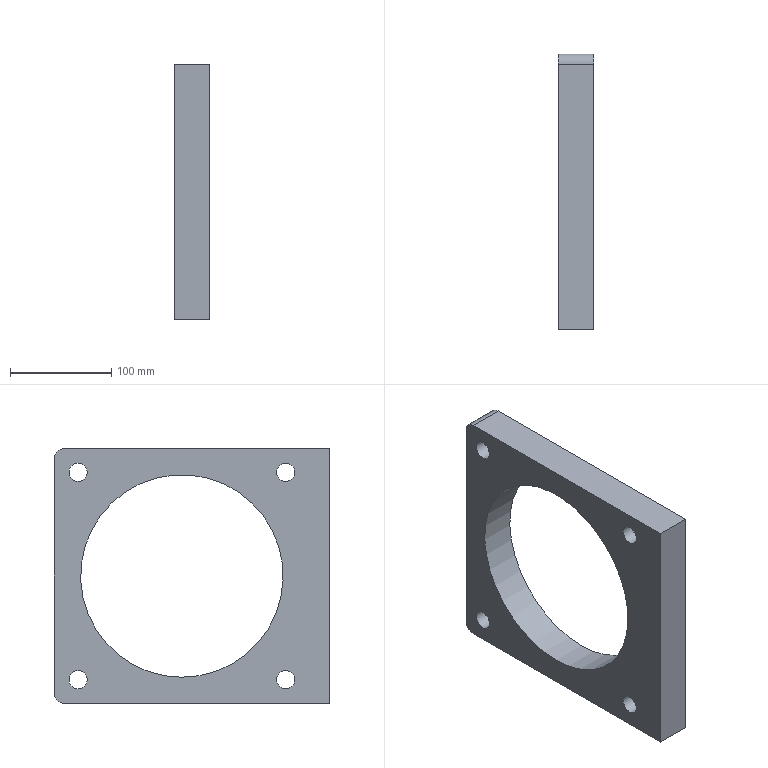Part | NX | features BREP 1, DATUM_CSYS 1 | 1 solid | 13 faces | box 35 x 272 x 252 mm | volume 1262355 mm3 | cylinder 7 | plane 6 | commonest cylinder face diameters 18 x4 20 x2 200 x1
STEP:
#1=CARTESIAN_POINT('',(-284.,116.,126.));
#2=VERTEX_POINT('',#1);
#3=CARTESIAN_POINT('',(-284.,-146.,126.));
#4=VERTEX_POINT('',#3);
#5=CARTESIAN_POINT('',(-284.,126.,126.));
#6=DIRECTION('',(0.,-1.,0.));
#7=VECTOR('',#6,1000.);
#8=LINE('',#5,#7);
#9=EDGE_CURVE('',#2,#4,#8,.T.);
#10=ORIENTED_EDGE('',*,*,#9,.F.);
#11=CARTESIAN_POINT('',(-319.,116.,126.));
#12=VERTEX_POINT('',#11);
#13=CARTESIAN_POINT('',(-284.,116.,126.));
#14=DIRECTION('',(-1.,0.,0.));
#15=VECTOR('',#14,1000.);
#16=LINE('',#13,#15);
#17=EDGE_CURVE('',#2,#12,#16,.T.);
#18=ORIENTED_EDGE('',*,*,#17,.T.);
#19=CARTESIAN_POINT('',(-319.,-146.,126.));
#20=VERTEX_POINT('',#19);
#21=CARTESIAN_POINT('',(-319.,126.,126.));
#22=DIRECTION('',(0.,-1.,0.));
#23=VECTOR('',#22,1000.);
#24=LINE('',#21,#23);
#25=EDGE_CURVE('',#12,#20,#24,.T.);
#26=ORIENTED_EDGE('',*,*,#25,.T.);
#27=CARTESIAN_POINT('',(-284.,-146.,126.));
#28=DIRECTION('',(-1.,0.,0.));
#29=VECTOR('',#28,1000.);
#30=LINE('',#27,#29);
#31=EDGE_CURVE('',#4,#20,#30,.T.);
#32=ORIENTED_EDGE('',*,*,#31,.F.);
#33=EDGE_LOOP('',(#10,#18,#26,#32));
#34=FACE_BOUND('',#33,.T.);
#35=CARTESIAN_POINT('',(-284.,126.,126.));
#36=DIRECTION('',(0.,0.,-1.));
#37=DIRECTION('',(0.,1.,0.));
#38=AXIS2_PLACEMENT_3D('',#35,#36,#37);
#39=PLANE('',#38);
#40=ADVANCED_FACE('',(#34),#39,.F.);
#41=CARTESIAN_POINT('',(-319.,-146.,-126.));
#42=VERTEX_POINT('',#41);
#43=CARTESIAN_POINT('',(-319.,-146.,126.));
#44=DIRECTION('',(0.,0.,-1.));
#45=VECTOR('',#44,1000.);
#46=LINE('',#43,#45);
#47=EDGE_CURVE('',#20,#42,#46,.T.);
#48=ORIENTED_EDGE('',*,*,#47,.T.);
#49=CARTESIAN_POINT('',(-284.,-146.,-126.));
#50=VERTEX_POINT('',#49);
#51=CARTESIAN_POINT('',(-284.,-146.,-126.));
#52=DIRECTION('',(-1.,0.,0.));
#53=VECTOR('',#52,1000.);
#54=LINE('',#51,#53);
#55=EDGE_CURVE('',#50,#42,#54,.T.);
#56=ORIENTED_EDGE('',*,*,#55,.F.);
#57=CARTESIAN_POINT('',(-284.,-146.,126.));
#58=DIRECTION('',(0.,0.,-1.));
#59=VECTOR('',#58,1000.);
#60=LINE('',#57,#59);
#61=EDGE_CURVE('',#4,#50,#60,.T.);
#62=ORIENTED_EDGE('',*,*,#61,.F.);
#63=ORIENTED_EDGE('',*,*,#31,.T.);
#64=EDGE_LOOP('',(#48,#56,#62,#63));
#65=FACE_BOUND('',#64,.T.);
#66=CARTESIAN_POINT('',(-284.,-146.,126.));
#67=DIRECTION('',(0.,1.,0.));
#68=DIRECTION('',(0.,0.,1.));
#69=AXIS2_PLACEMENT_3D('',#66,#67,#68);
#70=PLANE('',#69);
#71=ADVANCED_FACE('',(#65),#70,.F.);
#72=CARTESIAN_POINT('',(-319.,116.,-126.));
#73=VERTEX_POINT('',#72);
#74=CARTESIAN_POINT('',(-319.,-146.,-126.));
#75=DIRECTION('',(0.,1.,0.));
#76=VECTOR('',#75,1000.);
#77=LINE('',#74,#76);
#78=EDGE_CURVE('',#42,#73,#77,.T.);
#79=ORIENTED_EDGE('',*,*,#78,.T.);
#80=CARTESIAN_POINT('',(-284.,116.,-126.));
#81=VERTEX_POINT('',#80);
#82=CARTESIAN_POINT('',(-284.,116.,-126.));
#83=DIRECTION('',(-1.,0.,0.));
#84=VECTOR('',#83,1000.);
#85=LINE('',#82,#84);
#86=EDGE_CURVE('',#73,#81,#85,.F.);
#87=ORIENTED_EDGE('',*,*,#86,.T.);
#88=CARTESIAN_POINT('',(-284.,-146.,-126.));
#89=DIRECTION('',(0.,1.,0.));
#90=VECTOR('',#89,1000.);
#91=LINE('',#88,#90);
#92=EDGE_CURVE('',#50,#81,#91,.T.);
#93=ORIENTED_EDGE('',*,*,#92,.F.);
#94=ORIENTED_EDGE('',*,*,#55,.T.);
#95=EDGE_LOOP('',(#79,#87,#93,#94));
#96=FACE_BOUND('',#95,.T.);
#97=CARTESIAN_POINT('',(-284.,-146.,-126.));
#98=DIRECTION('',(0.,0.,1.));
#99=DIRECTION('',(1.,0.,0.));
#100=AXIS2_PLACEMENT_3D('',#97,#98,#99);
#101=PLANE('',#100);
#102=ADVANCED_FACE('',(#96),#101,.F.);
#103=CARTESIAN_POINT('',(-284.,126.,-116.));
#104=VERTEX_POINT('',#103);
#105=CARTESIAN_POINT('',(-284.,126.,116.));
#106=VERTEX_POINT('',#105);
#107=CARTESIAN_POINT('',(-284.,126.,-126.));
#108=DIRECTION('',(0.,0.,1.));
#109=VECTOR('',#108,1000.);
#110=LINE('',#107,#109);
#111=EDGE_CURVE('',#104,#106,#110,.T.);
#112=ORIENTED_EDGE('',*,*,#111,.F.);
#113=CARTESIAN_POINT('',(-319.,126.,-116.));
#114=VERTEX_POINT('',#113);
#115=CARTESIAN_POINT('',(-284.,126.,-116.));
#116=DIRECTION('',(-1.,0.,0.));
#117=VECTOR('',#116,1000.);
#118=LINE('',#115,#117);
#119=EDGE_CURVE('',#104,#114,#118,.T.);
#120=ORIENTED_EDGE('',*,*,#119,.T.);
#121=CARTESIAN_POINT('',(-319.,126.,116.));
#122=VERTEX_POINT('',#121);
#123=CARTESIAN_POINT('',(-319.,126.,-126.));
#124=DIRECTION('',(0.,0.,1.));
#125=VECTOR('',#124,1000.);
#126=LINE('',#123,#125);
#127=EDGE_CURVE('',#114,#122,#126,.T.);
#128=ORIENTED_EDGE('',*,*,#127,.T.);
#129=CARTESIAN_POINT('',(-284.,126.,116.));
#130=DIRECTION('',(-1.,0.,0.));
#131=VECTOR('',#130,1000.);
#132=LINE('',#129,#131);
#133=EDGE_CURVE('',#122,#106,#132,.F.);
#134=ORIENTED_EDGE('',*,*,#133,.T.);
#135=EDGE_LOOP('',(#112,#120,#128,#134));
#136=FACE_BOUND('',#135,.T.);
#137=CARTESIAN_POINT('',(-284.,126.,-126.));
#138=DIRECTION('',(0.,-1.,0.));
#139=DIRECTION('',(0.,0.,-1.));
#140=AXIS2_PLACEMENT_3D('',#137,#138,#139);
#141=PLANE('',#140);
#142=ADVANCED_FACE('',(#136),#141,.F.);
#143=CARTESIAN_POINT('',(-284.,0.,-100.));
#144=VERTEX_POINT('',#143);
#145=CARTESIAN_POINT('',(-284.,0.,0.));
#146=DIRECTION('',(1.,0.,0.));
#147=DIRECTION('',(0.,0.,-1.));
#148=AXIS2_PLACEMENT_3D('',#145,#146,#147);
#149=CIRCLE('',#148,100.);
#150=EDGE_CURVE('',#144,#144,#149,.T.);
#151=ORIENTED_EDGE('',*,*,#150,.F.);
#152=EDGE_LOOP('',(#151));
#153=FACE_BOUND('',#152,.T.);
#154=CARTESIAN_POINT('',(-284.,102.53,93.53));
#155=VERTEX_POINT('',#154);
#156=CARTESIAN_POINT('',(-284.,102.53,102.53));
#157=DIRECTION('',(1.,0.,0.));
#158=DIRECTION('',(0.,0.,-1.));
#159=AXIS2_PLACEMENT_3D('',#156,#157,#158);
#160=CIRCLE('',#159,9.);
#161=EDGE_CURVE('',#155,#155,#160,.T.);
#162=ORIENTED_EDGE('',*,*,#161,.F.);
#163=EDGE_LOOP('',(#162));
#164=FACE_BOUND('',#163,.T.);
#165=CARTESIAN_POINT('',(-284.,102.53,-111.53));
#166=VERTEX_POINT('',#165);
#167=CARTESIAN_POINT('',(-284.,102.53,-102.53));
#168=DIRECTION('',(1.,0.,0.));
#169=DIRECTION('',(0.,0.,-1.));
#170=AXIS2_PLACEMENT_3D('',#167,#168,#169);
#171=CIRCLE('',#170,9.);
#172=EDGE_CURVE('',#166,#166,#171,.T.);
#173=ORIENTED_EDGE('',*,*,#172,.F.);
#174=EDGE_LOOP('',(#173));
#175=FACE_BOUND('',#174,.T.);
#176=CARTESIAN_POINT('',(-284.,-102.53,93.53));
#177=VERTEX_POINT('',#176);
#178=CARTESIAN_POINT('',(-284.,-102.53,102.53));
#179=DIRECTION('',(1.,0.,0.));
#180=DIRECTION('',(0.,0.,-1.));
#181=AXIS2_PLACEMENT_3D('',#178,#179,#180);
#182=CIRCLE('',#181,9.);
#183=EDGE_CURVE('',#177,#177,#182,.T.);
#184=ORIENTED_EDGE('',*,*,#183,.F.);
#185=EDGE_LOOP('',(#184));
#186=FACE_BOUND('',#185,.T.);
#187=CARTESIAN_POINT('',(-284.,-102.53,-111.53));
#188=VERTEX_POINT('',#187);
#189=CARTESIAN_POINT('',(-284.,-102.53,-102.53));
#190=DIRECTION('',(1.,0.,0.));
#191=DIRECTION('',(0.,0.,-1.));
#192=AXIS2_PLACEMENT_3D('',#189,#190,#191);
#193=CIRCLE('',#192,9.);
#194=EDGE_CURVE('',#188,#188,#193,.T.);
#195=ORIENTED_EDGE('',*,*,#194,.F.);
#196=EDGE_LOOP('',(#195));
#197=FACE_BOUND('',#196,.T.);
#198=ORIENTED_EDGE('',*,*,#92,.T.);
#199=CARTESIAN_POINT('',(-284.,116.,-116.));
#200=DIRECTION('',(1.,0.,0.));
#201=DIRECTION('',(0.,0.,-1.));
#202=AXIS2_PLACEMENT_3D('',#199,#200,#201);
#203=CIRCLE('',#202,10.);
#204=EDGE_CURVE('',#81,#104,#203,.T.);
#205=ORIENTED_EDGE('',*,*,#204,.T.);
#206=ORIENTED_EDGE('',*,*,#111,.T.);
#207=CARTESIAN_POINT('',(-284.,116.,116.));
#208=DIRECTION('',(1.,0.,0.));
#209=DIRECTION('',(0.,0.,-1.));
#210=AXIS2_PLACEMENT_3D('',#207,#208,#209);
#211=CIRCLE('',#210,10.);
#212=EDGE_CURVE('',#106,#2,#211,.T.);
#213=ORIENTED_EDGE('',*,*,#212,.T.);
#214=ORIENTED_EDGE('',*,*,#9,.T.);
#215=ORIENTED_EDGE('',*,*,#61,.T.);
#216=EDGE_LOOP('',(#198,#205,#206,#213,#214,#215));
#217=FACE_BOUND('',#216,.T.);
#218=CARTESIAN_POINT('',(-284.,0.,0.));
#219=DIRECTION('',(1.,0.,0.));
#220=DIRECTION('',(0.,0.,-1.));
#221=AXIS2_PLACEMENT_3D('',#218,#219,#220);
#222=PLANE('',#221);
#223=ADVANCED_FACE('',(#153,#164,#175,#186,#197,#217),#222,.T.);
#224=CARTESIAN_POINT('',(-319.,0.,-100.));
#225=VERTEX_POINT('',#224);
#226=CARTESIAN_POINT('',(-319.,0.,0.));
#227=DIRECTION('',(1.,0.,0.));
#228=DIRECTION('',(0.,0.,-1.));
#229=AXIS2_PLACEMENT_3D('',#226,#227,#228);
#230=CIRCLE('',#229,100.);
#231=EDGE_CURVE('',#225,#225,#230,.T.);
#232=ORIENTED_EDGE('',*,*,#231,.T.);
#233=EDGE_LOOP('',(#232));
#234=FACE_BOUND('',#233,.T.);
#235=CARTESIAN_POINT('',(-319.,102.53,93.53));
#236=VERTEX_POINT('',#235);
#237=CARTESIAN_POINT('',(-319.,102.53,102.53));
#238=DIRECTION('',(1.,0.,0.));
#239=DIRECTION('',(0.,0.,-1.));
#240=AXIS2_PLACEMENT_3D('',#237,#238,#239);
#241=CIRCLE('',#240,9.);
#242=EDGE_CURVE('',#236,#236,#241,.T.);
#243=ORIENTED_EDGE('',*,*,#242,.T.);
#244=EDGE_LOOP('',(#243));
#245=FACE_BOUND('',#244,.T.);
#246=CARTESIAN_POINT('',(-319.,102.53,-111.53));
#247=VERTEX_POINT('',#246);
#248=CARTESIAN_POINT('',(-319.,102.53,-102.53));
#249=DIRECTION('',(1.,0.,0.));
#250=DIRECTION('',(0.,0.,-1.));
#251=AXIS2_PLACEMENT_3D('',#248,#249,#250);
#252=CIRCLE('',#251,9.);
#253=EDGE_CURVE('',#247,#247,#252,.T.);
#254=ORIENTED_EDGE('',*,*,#253,.T.);
#255=EDGE_LOOP('',(#254));
#256=FACE_BOUND('',#255,.T.);
#257=CARTESIAN_POINT('',(-319.,-102.53,93.53));
#258=VERTEX_POINT('',#257);
#259=CARTESIAN_POINT('',(-319.,-102.53,102.53));
#260=DIRECTION('',(1.,0.,0.));
#261=DIRECTION('',(0.,0.,-1.));
#262=AXIS2_PLACEMENT_3D('',#259,#260,#261);
#263=CIRCLE('',#262,9.);
#264=EDGE_CURVE('',#258,#258,#263,.T.);
#265=ORIENTED_EDGE('',*,*,#264,.T.);
#266=EDGE_LOOP('',(#265));
#267=FACE_BOUND('',#266,.T.);
#268=CARTESIAN_POINT('',(-319.,-102.53,-111.53));
#269=VERTEX_POINT('',#268);
#270=CARTESIAN_POINT('',(-319.,-102.53,-102.53));
#271=DIRECTION('',(1.,0.,0.));
#272=DIRECTION('',(0.,0.,-1.));
#273=AXIS2_PLACEMENT_3D('',#270,#271,#272);
#274=CIRCLE('',#273,9.);
#275=EDGE_CURVE('',#269,#269,#274,.T.);
#276=ORIENTED_EDGE('',*,*,#275,.T.);
#277=EDGE_LOOP('',(#276));
#278=FACE_BOUND('',#277,.T.);
#279=ORIENTED_EDGE('',*,*,#127,.F.);
#280=CARTESIAN_POINT('',(-319.,116.,-116.));
#281=DIRECTION('',(1.,0.,0.));
#282=DIRECTION('',(0.,0.,-1.));
#283=AXIS2_PLACEMENT_3D('',#280,#281,#282);
#284=CIRCLE('',#283,10.);
#285=EDGE_CURVE('',#114,#73,#284,.F.);
#286=ORIENTED_EDGE('',*,*,#285,.T.);
#287=ORIENTED_EDGE('',*,*,#78,.F.);
#288=ORIENTED_EDGE('',*,*,#47,.F.);
#289=ORIENTED_EDGE('',*,*,#25,.F.);
#290=CARTESIAN_POINT('',(-319.,116.,116.));
#291=DIRECTION('',(1.,0.,0.));
#292=DIRECTION('',(0.,0.,-1.));
#293=AXIS2_PLACEMENT_3D('',#290,#291,#292);
#294=CIRCLE('',#293,10.);
#295=EDGE_CURVE('',#12,#122,#294,.F.);
#296=ORIENTED_EDGE('',*,*,#295,.T.);
#297=EDGE_LOOP('',(#279,#286,#287,#288,#289,#296));
#298=FACE_BOUND('',#297,.T.);
#299=CARTESIAN_POINT('',(-319.,0.,0.));
#300=DIRECTION('',(1.,0.,0.));
#301=DIRECTION('',(0.,0.,-1.));
#302=AXIS2_PLACEMENT_3D('',#299,#300,#301);
#303=PLANE('',#302);
#304=ADVANCED_FACE('',(#234,#245,#256,#267,#278,#298),#303,.F.);
#305=ORIENTED_EDGE('',*,*,#204,.F.);
#306=ORIENTED_EDGE('',*,*,#86,.F.);
#307=ORIENTED_EDGE('',*,*,#285,.F.);
#308=ORIENTED_EDGE('',*,*,#119,.F.);
#309=EDGE_LOOP('',(#305,#306,#307,#308));
#310=FACE_BOUND('',#309,.T.);
#311=CARTESIAN_POINT('',(-284.,116.,-116.));
#312=DIRECTION('',(-1.,0.,0.));
#313=DIRECTION('',(0.,0.,1.));
#314=AXIS2_PLACEMENT_3D('',#311,#312,#313);
#315=CYLINDRICAL_SURFACE('',#314,10.);
#316=ADVANCED_FACE('',(#310),#315,.T.);
#317=ORIENTED_EDGE('',*,*,#212,.F.);
#318=ORIENTED_EDGE('',*,*,#133,.F.);
#319=ORIENTED_EDGE('',*,*,#295,.F.);
#320=ORIENTED_EDGE('',*,*,#17,.F.);
#321=EDGE_LOOP('',(#317,#318,#319,#320));
#322=FACE_BOUND('',#321,.T.);
#323=CARTESIAN_POINT('',(-284.,116.,116.));
#324=DIRECTION('',(-1.,0.,0.));
#325=DIRECTION('',(0.,0.,1.));
#326=AXIS2_PLACEMENT_3D('',#323,#324,#325);
#327=CYLINDRICAL_SURFACE('',#326,10.);
#328=ADVANCED_FACE('',(#322),#327,.T.);
#329=ORIENTED_EDGE('',*,*,#194,.T.);
#330=EDGE_LOOP('',(#329));
#331=FACE_BOUND('',#330,.T.);
#332=ORIENTED_EDGE('',*,*,#275,.F.);
#333=EDGE_LOOP('',(#332));
#334=FACE_BOUND('',#333,.T.);
#335=CARTESIAN_POINT('',(-319.,-102.53,-102.53));
#336=DIRECTION('',(1.,0.,0.));
#337=DIRECTION('',(0.,0.,-1.));
#338=AXIS2_PLACEMENT_3D('',#335,#336,#337);
#339=CYLINDRICAL_SURFACE('',#338,9.);
#340=ADVANCED_FACE('',(#331,#334),#339,.F.);
#341=ORIENTED_EDGE('',*,*,#183,.T.);
#342=EDGE_LOOP('',(#341));
#343=FACE_BOUND('',#342,.T.);
#344=ORIENTED_EDGE('',*,*,#264,.F.);
#345=EDGE_LOOP('',(#344));
#346=FACE_BOUND('',#345,.T.);
#347=CARTESIAN_POINT('',(-319.,-102.53,102.53));
#348=DIRECTION('',(1.,0.,0.));
#349=DIRECTION('',(0.,0.,-1.));
#350=AXIS2_PLACEMENT_3D('',#347,#348,#349);
#351=CYLINDRICAL_SURFACE('',#350,9.);
#352=ADVANCED_FACE('',(#343,#346),#351,.F.);
#353=ORIENTED_EDGE('',*,*,#172,.T.);
#354=EDGE_LOOP('',(#353));
#355=FACE_BOUND('',#354,.T.);
#356=ORIENTED_EDGE('',*,*,#253,.F.);
#357=EDGE_LOOP('',(#356));
#358=FACE_BOUND('',#357,.T.);
#359=CARTESIAN_POINT('',(-319.,102.53,-102.53));
#360=DIRECTION('',(1.,0.,0.));
#361=DIRECTION('',(0.,0.,-1.));
#362=AXIS2_PLACEMENT_3D('',#359,#360,#361);
#363=CYLINDRICAL_SURFACE('',#362,9.);
#364=ADVANCED_FACE('',(#355,#358),#363,.F.);
#365=ORIENTED_EDGE('',*,*,#161,.T.);
#366=EDGE_LOOP('',(#365));
#367=FACE_BOUND('',#366,.T.);
#368=ORIENTED_EDGE('',*,*,#242,.F.);
#369=EDGE_LOOP('',(#368));
#370=FACE_BOUND('',#369,.T.);
#371=CARTESIAN_POINT('',(-319.,102.53,102.53));
#372=DIRECTION('',(1.,0.,0.));
#373=DIRECTION('',(0.,0.,-1.));
#374=AXIS2_PLACEMENT_3D('',#371,#372,#373);
#375=CYLINDRICAL_SURFACE('',#374,9.);
#376=ADVANCED_FACE('',(#367,#370),#375,.F.);
#377=ORIENTED_EDGE('',*,*,#150,.T.);
#378=EDGE_LOOP('',(#377));
#379=FACE_BOUND('',#378,.T.);
#380=ORIENTED_EDGE('',*,*,#231,.F.);
#381=EDGE_LOOP('',(#380));
#382=FACE_BOUND('',#381,.T.);
#383=CARTESIAN_POINT('',(-319.,0.,0.));
#384=DIRECTION('',(1.,0.,0.));
#385=DIRECTION('',(0.,0.,-1.));
#386=AXIS2_PLACEMENT_3D('',#383,#384,#385);
#387=CYLINDRICAL_SURFACE('',#386,100.);
#388=ADVANCED_FACE('',(#379,#382),#387,.F.);
#389=CLOSED_SHELL('',(#40,#71,#102,#142,#223,#304,#316,#328,#340,#352,#364,#376,#388));
#390=MANIFOLD_SOLID_BREP('',#389);
#391=(LENGTH_UNIT()NAMED_UNIT(*)SI_UNIT(.MILLI.,.METRE.));
#392=UNCERTAINTY_MEASURE_WITH_UNIT(LENGTH_MEASURE(0.00001),#391,'','');
#393=(NAMED_UNIT(*)PLANE_ANGLE_UNIT()SI_UNIT($,.RADIAN.));
#394=(NAMED_UNIT(*)SI_UNIT($,.STERADIAN.)SOLID_ANGLE_UNIT());
#395=(GEOMETRIC_REPRESENTATION_CONTEXT(3)GLOBAL_UNCERTAINTY_ASSIGNED_CONTEXT((#392))GLOBAL_UNIT_ASSIGNED_CONTEXT((#391,#393,#394))REPRESENTATION_CONTEXT('',''));
#396=ADVANCED_BREP_SHAPE_REPRESENTATION('',(#390),#395);